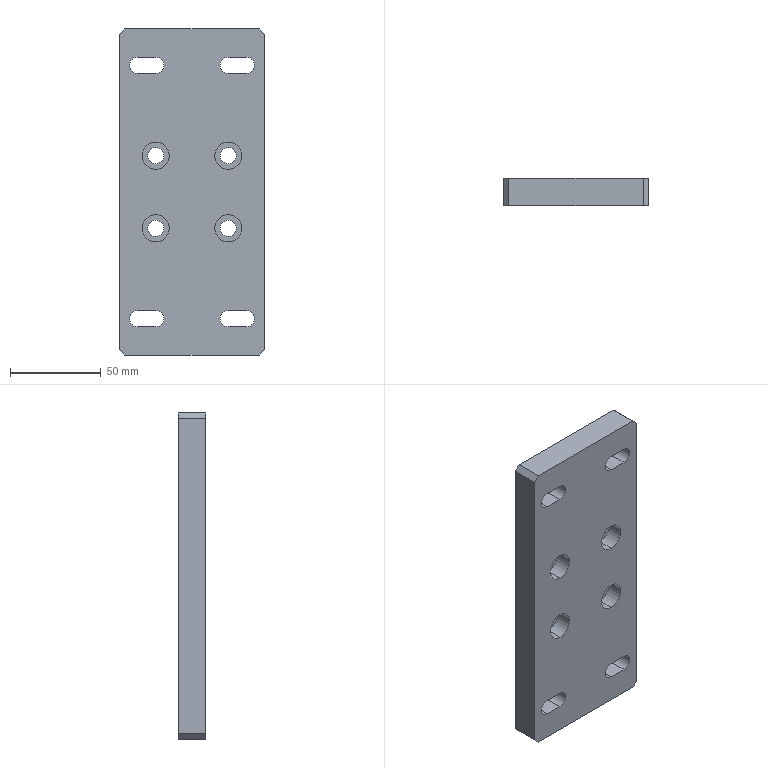Part | SolidWorks | features BaseBody 1 | 1 solid | 46 faces | box 80 x 15 x 180 mm | volume 198624 mm3 | cylinder 24 | plane 22 | commonest cylinder face diameters 9 x16 15 x8
STEP:
#1=CARTESIAN_POINT('',(-40.,7.5,87.));
#2=VERTEX_POINT('',#1);
#3=CARTESIAN_POINT('',(-37.,7.5,90.));
#4=VERTEX_POINT('',#3);
#5=CARTESIAN_POINT('',(-37.,7.5,90.));
#6=DIRECTION('',(0.7071,0.,0.7071));
#7=VECTOR('',#6,1000.);
#8=LINE('',#5,#7);
#9=EDGE_CURVE('',#2,#4,#8,.T.);
#10=ORIENTED_EDGE('',*,*,#9,.F.);
#11=CARTESIAN_POINT('',(-40.,-7.5,87.));
#12=VERTEX_POINT('',#11);
#13=CARTESIAN_POINT('',(-40.,7.5,87.));
#14=DIRECTION('',(0.,1.,0.));
#15=VECTOR('',#14,1000.);
#16=LINE('',#13,#15);
#17=EDGE_CURVE('',#12,#2,#16,.T.);
#18=ORIENTED_EDGE('',*,*,#17,.F.);
#19=CARTESIAN_POINT('',(-37.,-7.5,90.));
#20=VERTEX_POINT('',#19);
#21=CARTESIAN_POINT('',(-63.5,-7.5,63.5));
#22=DIRECTION('',(-0.7071,0.,-0.7071));
#23=VECTOR('',#22,1000.);
#24=LINE('',#21,#23);
#25=EDGE_CURVE('',#20,#12,#24,.T.);
#26=ORIENTED_EDGE('',*,*,#25,.F.);
#27=CARTESIAN_POINT('',(-37.,7.5,90.));
#28=DIRECTION('',(0.,-1.,0.));
#29=VECTOR('',#28,1000.);
#30=LINE('',#27,#29);
#31=EDGE_CURVE('',#4,#20,#30,.T.);
#32=ORIENTED_EDGE('',*,*,#31,.F.);
#33=EDGE_LOOP('',(#10,#18,#26,#32));
#34=FACE_OUTER_BOUND('',#33,.T.);
#35=CARTESIAN_POINT('',(-37.,7.5,90.));
#36=DIRECTION('',(0.7071,0.,-0.7071));
#37=DIRECTION('',(0.,-1.,0.));
#38=AXIS2_PLACEMENT_3D('',#35,#36,#37);
#39=PLANE('',#38);
#40=ADVANCED_FACE('',(#34),#39,.F.);
#41=CARTESIAN_POINT('',(-37.,7.5,-90.));
#42=VERTEX_POINT('',#41);
#43=CARTESIAN_POINT('',(-40.,7.5,-87.));
#44=VERTEX_POINT('',#43);
#45=CARTESIAN_POINT('',(-40.,7.5,-87.));
#46=DIRECTION('',(-0.7071,0.,0.7071));
#47=VECTOR('',#46,1000.);
#48=LINE('',#45,#47);
#49=EDGE_CURVE('',#42,#44,#48,.T.);
#50=ORIENTED_EDGE('',*,*,#49,.F.);
#51=CARTESIAN_POINT('',(-37.,-7.5,-90.));
#52=VERTEX_POINT('',#51);
#53=CARTESIAN_POINT('',(-37.,7.5,-90.));
#54=DIRECTION('',(0.,1.,0.));
#55=VECTOR('',#54,1000.);
#56=LINE('',#53,#55);
#57=EDGE_CURVE('',#52,#42,#56,.T.);
#58=ORIENTED_EDGE('',*,*,#57,.F.);
#59=CARTESIAN_POINT('',(-40.,-7.5,-87.));
#60=VERTEX_POINT('',#59);
#61=CARTESIAN_POINT('',(-63.5,-7.5,-63.5));
#62=DIRECTION('',(0.7071,0.,-0.7071));
#63=VECTOR('',#62,1000.);
#64=LINE('',#61,#63);
#65=EDGE_CURVE('',#60,#52,#64,.T.);
#66=ORIENTED_EDGE('',*,*,#65,.F.);
#67=CARTESIAN_POINT('',(-40.,7.5,-87.));
#68=DIRECTION('',(0.,-1.,0.));
#69=VECTOR('',#68,1000.);
#70=LINE('',#67,#69);
#71=EDGE_CURVE('',#44,#60,#70,.T.);
#72=ORIENTED_EDGE('',*,*,#71,.F.);
#73=EDGE_LOOP('',(#50,#58,#66,#72));
#74=FACE_OUTER_BOUND('',#73,.T.);
#75=CARTESIAN_POINT('',(-40.,7.5,-87.));
#76=DIRECTION('',(0.7071,0.,0.7071));
#77=DIRECTION('',(0.,-1.,0.));
#78=AXIS2_PLACEMENT_3D('',#75,#76,#77);
#79=PLANE('',#78);
#80=ADVANCED_FACE('',(#74),#79,.F.);
#81=CARTESIAN_POINT('',(37.,7.5,90.));
#82=VERTEX_POINT('',#81);
#83=CARTESIAN_POINT('',(40.,7.5,87.));
#84=VERTEX_POINT('',#83);
#85=CARTESIAN_POINT('',(40.,7.5,87.));
#86=DIRECTION('',(0.7071,0.,-0.7071));
#87=VECTOR('',#86,1000.);
#88=LINE('',#85,#87);
#89=EDGE_CURVE('',#82,#84,#88,.T.);
#90=ORIENTED_EDGE('',*,*,#89,.F.);
#91=CARTESIAN_POINT('',(37.,-7.5,90.));
#92=VERTEX_POINT('',#91);
#93=CARTESIAN_POINT('',(37.,7.5,90.));
#94=DIRECTION('',(0.,1.,0.));
#95=VECTOR('',#94,1000.);
#96=LINE('',#93,#95);
#97=EDGE_CURVE('',#92,#82,#96,.T.);
#98=ORIENTED_EDGE('',*,*,#97,.F.);
#99=CARTESIAN_POINT('',(40.,-7.5,87.));
#100=VERTEX_POINT('',#99);
#101=CARTESIAN_POINT('',(63.5,-7.5,63.5));
#102=DIRECTION('',(-0.7071,0.,0.7071));
#103=VECTOR('',#102,1000.);
#104=LINE('',#101,#103);
#105=EDGE_CURVE('',#100,#92,#104,.T.);
#106=ORIENTED_EDGE('',*,*,#105,.F.);
#107=CARTESIAN_POINT('',(40.,7.5,87.));
#108=DIRECTION('',(0.,-1.,0.));
#109=VECTOR('',#108,1000.);
#110=LINE('',#107,#109);
#111=EDGE_CURVE('',#84,#100,#110,.T.);
#112=ORIENTED_EDGE('',*,*,#111,.F.);
#113=EDGE_LOOP('',(#90,#98,#106,#112));
#114=FACE_OUTER_BOUND('',#113,.T.);
#115=CARTESIAN_POINT('',(40.,7.5,87.));
#116=DIRECTION('',(-0.7071,0.,-0.7071));
#117=DIRECTION('',(-0.7071,0.,0.7071));
#118=AXIS2_PLACEMENT_3D('',#115,#116,#117);
#119=PLANE('',#118);
#120=ADVANCED_FACE('',(#114),#119,.F.);
#121=CARTESIAN_POINT('',(40.,7.5,-87.));
#122=VERTEX_POINT('',#121);
#123=CARTESIAN_POINT('',(37.,7.5,-90.));
#124=VERTEX_POINT('',#123);
#125=CARTESIAN_POINT('',(37.,7.5,-90.));
#126=DIRECTION('',(-0.7071,0.,-0.7071));
#127=VECTOR('',#126,1000.);
#128=LINE('',#125,#127);
#129=EDGE_CURVE('',#122,#124,#128,.T.);
#130=ORIENTED_EDGE('',*,*,#129,.F.);
#131=CARTESIAN_POINT('',(40.,-7.5,-87.));
#132=VERTEX_POINT('',#131);
#133=CARTESIAN_POINT('',(40.,7.5,-87.));
#134=DIRECTION('',(0.,1.,0.));
#135=VECTOR('',#134,1000.);
#136=LINE('',#133,#135);
#137=EDGE_CURVE('',#132,#122,#136,.T.);
#138=ORIENTED_EDGE('',*,*,#137,.F.);
#139=CARTESIAN_POINT('',(37.,-7.5,-90.));
#140=VERTEX_POINT('',#139);
#141=CARTESIAN_POINT('',(63.5,-7.5,-63.5));
#142=DIRECTION('',(0.7071,0.,0.7071));
#143=VECTOR('',#142,1000.);
#144=LINE('',#141,#143);
#145=EDGE_CURVE('',#140,#132,#144,.T.);
#146=ORIENTED_EDGE('',*,*,#145,.F.);
#147=CARTESIAN_POINT('',(37.,7.5,-90.));
#148=DIRECTION('',(0.,-1.,0.));
#149=VECTOR('',#148,1000.);
#150=LINE('',#147,#149);
#151=EDGE_CURVE('',#124,#140,#150,.T.);
#152=ORIENTED_EDGE('',*,*,#151,.F.);
#153=EDGE_LOOP('',(#130,#138,#146,#152));
#154=FACE_OUTER_BOUND('',#153,.T.);
#155=CARTESIAN_POINT('',(37.,7.5,-90.));
#156=DIRECTION('',(-0.7071,0.,0.7071));
#157=DIRECTION('',(0.,1.,0.));
#158=AXIS2_PLACEMENT_3D('',#155,#156,#157);
#159=PLANE('',#158);
#160=ADVANCED_FACE('',(#154),#159,.F.);
#161=CARTESIAN_POINT('',(-20.,-7.5,74.5));
#162=VERTEX_POINT('',#161);
#163=CARTESIAN_POINT('',(-30.,-7.5,74.5));
#164=VERTEX_POINT('',#163);
#165=CARTESIAN_POINT('',(0.,-7.5,74.5));
#166=DIRECTION('',(-1.,0.,0.));
#167=VECTOR('',#166,1000.);
#168=LINE('',#165,#167);
#169=EDGE_CURVE('',#162,#164,#168,.T.);
#170=ORIENTED_EDGE('',*,*,#169,.T.);
#171=CARTESIAN_POINT('',(-30.,7.5,74.5));
#172=VERTEX_POINT('',#171);
#173=CARTESIAN_POINT('',(-30.,7.5,74.5));
#174=DIRECTION('',(0.,1.,0.));
#175=VECTOR('',#174,1000.);
#176=LINE('',#173,#175);
#177=EDGE_CURVE('',#164,#172,#176,.T.);
#178=ORIENTED_EDGE('',*,*,#177,.T.);
#179=CARTESIAN_POINT('',(-20.,7.5,74.5));
#180=VERTEX_POINT('',#179);
#181=CARTESIAN_POINT('',(-30.,7.5,74.5));
#182=DIRECTION('',(1.,0.,0.));
#183=VECTOR('',#182,1000.);
#184=LINE('',#181,#183);
#185=EDGE_CURVE('',#172,#180,#184,.T.);
#186=ORIENTED_EDGE('',*,*,#185,.T.);
#187=CARTESIAN_POINT('',(-20.,7.5,74.5));
#188=DIRECTION('',(0.,-1.,0.));
#189=VECTOR('',#188,1000.);
#190=LINE('',#187,#189);
#191=EDGE_CURVE('',#180,#162,#190,.T.);
#192=ORIENTED_EDGE('',*,*,#191,.T.);
#193=EDGE_LOOP('',(#170,#178,#186,#192));
#194=FACE_OUTER_BOUND('',#193,.T.);
#195=CARTESIAN_POINT('',(-30.,7.5,74.5));
#196=DIRECTION('',(0.,0.,1.));
#197=DIRECTION('',(1.,0.,0.));
#198=AXIS2_PLACEMENT_3D('',#195,#196,#197);
#199=PLANE('',#198);
#200=ADVANCED_FACE('',(#194),#199,.F.);
#201=CARTESIAN_POINT('',(-30.,-7.5,65.5));
#202=VERTEX_POINT('',#201);
#203=CARTESIAN_POINT('',(-20.,-7.5,65.5));
#204=VERTEX_POINT('',#203);
#205=CARTESIAN_POINT('',(0.,-7.5,65.5));
#206=DIRECTION('',(1.,0.,0.));
#207=VECTOR('',#206,1000.);
#208=LINE('',#205,#207);
#209=EDGE_CURVE('',#202,#204,#208,.T.);
#210=ORIENTED_EDGE('',*,*,#209,.T.);
#211=CARTESIAN_POINT('',(-20.,7.5,65.5));
#212=VERTEX_POINT('',#211);
#213=CARTESIAN_POINT('',(-20.,7.5,65.5));
#214=DIRECTION('',(0.,1.,0.));
#215=VECTOR('',#214,1000.);
#216=LINE('',#213,#215);
#217=EDGE_CURVE('',#204,#212,#216,.T.);
#218=ORIENTED_EDGE('',*,*,#217,.T.);
#219=CARTESIAN_POINT('',(-30.,7.5,65.5));
#220=VERTEX_POINT('',#219);
#221=CARTESIAN_POINT('',(-30.,7.5,65.5));
#222=DIRECTION('',(1.,0.,0.));
#223=VECTOR('',#222,1000.);
#224=LINE('',#221,#223);
#225=EDGE_CURVE('',#220,#212,#224,.T.);
#226=ORIENTED_EDGE('',*,*,#225,.F.);
#227=CARTESIAN_POINT('',(-30.,7.5,65.5));
#228=DIRECTION('',(0.,-1.,0.));
#229=VECTOR('',#228,1000.);
#230=LINE('',#227,#229);
#231=EDGE_CURVE('',#220,#202,#230,.T.);
#232=ORIENTED_EDGE('',*,*,#231,.T.);
#233=EDGE_LOOP('',(#210,#218,#226,#232));
#234=FACE_OUTER_BOUND('',#233,.T.);
#235=CARTESIAN_POINT('',(-30.,7.5,65.5));
#236=DIRECTION('',(0.,0.,-1.));
#237=DIRECTION('',(0.,-1.,0.));
#238=AXIS2_PLACEMENT_3D('',#235,#236,#237);
#239=PLANE('',#238);
#240=ADVANCED_FACE('',(#234),#239,.F.);
#241=CARTESIAN_POINT('',(-30.,-7.5,70.));
#242=DIRECTION('',(0.,-1.,0.));
#243=DIRECTION('',(0.,0.,-1.));
#244=AXIS2_PLACEMENT_3D('',#241,#242,#243);
#245=CIRCLE('',#244,4.5);
#246=EDGE_CURVE('',#164,#202,#245,.T.);
#247=ORIENTED_EDGE('',*,*,#246,.T.);
#248=ORIENTED_EDGE('',*,*,#231,.F.);
#249=CARTESIAN_POINT('',(-30.,7.5,70.));
#250=DIRECTION('',(0.,1.,0.));
#251=DIRECTION('',(0.,0.,1.));
#252=AXIS2_PLACEMENT_3D('',#249,#250,#251);
#253=CIRCLE('',#252,4.5);
#254=EDGE_CURVE('',#220,#172,#253,.T.);
#255=ORIENTED_EDGE('',*,*,#254,.T.);
#256=ORIENTED_EDGE('',*,*,#177,.F.);
#257=EDGE_LOOP('',(#247,#248,#255,#256));
#258=FACE_OUTER_BOUND('',#257,.T.);
#259=CARTESIAN_POINT('',(-30.,7.5,70.));
#260=DIRECTION('',(0.,1.,0.));
#261=DIRECTION('',(0.,0.,1.));
#262=AXIS2_PLACEMENT_3D('',#259,#260,#261);
#263=CYLINDRICAL_SURFACE('',#262,4.5);
#264=ADVANCED_FACE('',(#258),#263,.F.);
#265=CARTESIAN_POINT('',(-20.,-7.5,70.));
#266=DIRECTION('',(0.,-1.,0.));
#267=DIRECTION('',(0.,0.,-1.));
#268=AXIS2_PLACEMENT_3D('',#265,#266,#267);
#269=CIRCLE('',#268,4.5);
#270=EDGE_CURVE('',#204,#162,#269,.T.);
#271=ORIENTED_EDGE('',*,*,#270,.T.);
#272=ORIENTED_EDGE('',*,*,#191,.F.);
#273=CARTESIAN_POINT('',(-20.,7.5,70.));
#274=DIRECTION('',(0.,1.,0.));
#275=DIRECTION('',(0.,0.,1.));
#276=AXIS2_PLACEMENT_3D('',#273,#274,#275);
#277=CIRCLE('',#276,4.5);
#278=EDGE_CURVE('',#180,#212,#277,.T.);
#279=ORIENTED_EDGE('',*,*,#278,.T.);
#280=ORIENTED_EDGE('',*,*,#217,.F.);
#281=EDGE_LOOP('',(#271,#272,#279,#280));
#282=FACE_OUTER_BOUND('',#281,.T.);
#283=CARTESIAN_POINT('',(-20.,7.5,70.));
#284=DIRECTION('',(0.,1.,0.));
#285=DIRECTION('',(0.,0.,1.));
#286=AXIS2_PLACEMENT_3D('',#283,#284,#285);
#287=CYLINDRICAL_SURFACE('',#286,4.5);
#288=ADVANCED_FACE('',(#282),#287,.F.);
#289=CARTESIAN_POINT('',(30.,-7.5,74.5));
#290=VERTEX_POINT('',#289);
#291=CARTESIAN_POINT('',(20.,-7.5,74.5));
#292=VERTEX_POINT('',#291);
#293=CARTESIAN_POINT('',(0.,-7.5,74.5));
#294=DIRECTION('',(-1.,0.,0.));
#295=VECTOR('',#294,1000.);
#296=LINE('',#293,#295);
#297=EDGE_CURVE('',#290,#292,#296,.T.);
#298=ORIENTED_EDGE('',*,*,#297,.T.);
#299=CARTESIAN_POINT('',(20.,7.5,74.5));
#300=VERTEX_POINT('',#299);
#301=CARTESIAN_POINT('',(20.,7.5,74.5));
#302=DIRECTION('',(0.,1.,0.));
#303=VECTOR('',#302,1000.);
#304=LINE('',#301,#303);
#305=EDGE_CURVE('',#292,#300,#304,.T.);
#306=ORIENTED_EDGE('',*,*,#305,.T.);
#307=CARTESIAN_POINT('',(30.,7.5,74.5));
#308=VERTEX_POINT('',#307);
#309=CARTESIAN_POINT('',(20.,7.5,74.5));
#310=DIRECTION('',(1.,0.,0.));
#311=VECTOR('',#310,1000.);
#312=LINE('',#309,#311);
#313=EDGE_CURVE('',#300,#308,#312,.T.);
#314=ORIENTED_EDGE('',*,*,#313,.T.);
#315=CARTESIAN_POINT('',(30.,7.5,74.5));
#316=DIRECTION('',(0.,-1.,0.));
#317=VECTOR('',#316,1000.);
#318=LINE('',#315,#317);
#319=EDGE_CURVE('',#308,#290,#318,.T.);
#320=ORIENTED_EDGE('',*,*,#319,.T.);
#321=EDGE_LOOP('',(#298,#306,#314,#320));
#322=FACE_OUTER_BOUND('',#321,.T.);
#323=CARTESIAN_POINT('',(20.,7.5,74.5));
#324=DIRECTION('',(0.,0.,1.));
#325=DIRECTION('',(1.,0.,0.));
#326=AXIS2_PLACEMENT_3D('',#323,#324,#325);
#327=PLANE('',#326);
#328=ADVANCED_FACE('',(#322),#327,.F.);
#329=CARTESIAN_POINT('',(20.,-7.5,65.5));
#330=VERTEX_POINT('',#329);
#331=CARTESIAN_POINT('',(30.,-7.5,65.5));
#332=VERTEX_POINT('',#331);
#333=CARTESIAN_POINT('',(0.,-7.5,65.5));
#334=DIRECTION('',(1.,0.,0.));
#335=VECTOR('',#334,1000.);
#336=LINE('',#333,#335);
#337=EDGE_CURVE('',#330,#332,#336,.T.);
#338=ORIENTED_EDGE('',*,*,#337,.T.);
#339=CARTESIAN_POINT('',(30.,7.5,65.5));
#340=VERTEX_POINT('',#339);
#341=CARTESIAN_POINT('',(30.,7.5,65.5));
#342=DIRECTION('',(0.,1.,0.));
#343=VECTOR('',#342,1000.);
#344=LINE('',#341,#343);
#345=EDGE_CURVE('',#332,#340,#344,.T.);
#346=ORIENTED_EDGE('',*,*,#345,.T.);
#347=CARTESIAN_POINT('',(20.,7.5,65.5));
#348=VERTEX_POINT('',#347);
#349=CARTESIAN_POINT('',(20.,7.5,65.5));
#350=DIRECTION('',(1.,0.,0.));
#351=VECTOR('',#350,1000.);
#352=LINE('',#349,#351);
#353=EDGE_CURVE('',#348,#340,#352,.T.);
#354=ORIENTED_EDGE('',*,*,#353,.F.);
#355=CARTESIAN_POINT('',(20.,7.5,65.5));
#356=DIRECTION('',(0.,-1.,0.));
#357=VECTOR('',#356,1000.);
#358=LINE('',#355,#357);
#359=EDGE_CURVE('',#348,#330,#358,.T.);
#360=ORIENTED_EDGE('',*,*,#359,.T.);
#361=EDGE_LOOP('',(#338,#346,#354,#360));
#362=FACE_OUTER_BOUND('',#361,.T.);
#363=CARTESIAN_POINT('',(20.,7.5,65.5));
#364=DIRECTION('',(0.,0.,-1.));
#365=DIRECTION('',(0.,-1.,0.));
#366=AXIS2_PLACEMENT_3D('',#363,#364,#365);
#367=PLANE('',#366);
#368=ADVANCED_FACE('',(#362),#367,.F.);
#369=CARTESIAN_POINT('',(20.,-7.5,70.));
#370=DIRECTION('',(0.,-1.,0.));
#371=DIRECTION('',(0.,0.,-1.));
#372=AXIS2_PLACEMENT_3D('',#369,#370,#371);
#373=CIRCLE('',#372,4.5);
#374=EDGE_CURVE('',#292,#330,#373,.T.);
#375=ORIENTED_EDGE('',*,*,#374,.T.);
#376=ORIENTED_EDGE('',*,*,#359,.F.);
#377=CARTESIAN_POINT('',(20.,7.5,70.));
#378=DIRECTION('',(0.,1.,0.));
#379=DIRECTION('',(0.,0.,1.));
#380=AXIS2_PLACEMENT_3D('',#377,#378,#379);
#381=CIRCLE('',#380,4.5);
#382=EDGE_CURVE('',#348,#300,#381,.T.);
#383=ORIENTED_EDGE('',*,*,#382,.T.);
#384=ORIENTED_EDGE('',*,*,#305,.F.);
#385=EDGE_LOOP('',(#375,#376,#383,#384));
#386=FACE_OUTER_BOUND('',#385,.T.);
#387=CARTESIAN_POINT('',(20.,7.5,70.));
#388=DIRECTION('',(0.,1.,0.));
#389=DIRECTION('',(0.,0.,1.));
#390=AXIS2_PLACEMENT_3D('',#387,#388,#389);
#391=CYLINDRICAL_SURFACE('',#390,4.5);
#392=ADVANCED_FACE('',(#386),#391,.F.);
#393=CARTESIAN_POINT('',(30.,-7.5,70.));
#394=DIRECTION('',(0.,-1.,0.));
#395=DIRECTION('',(0.,0.,-1.));
#396=AXIS2_PLACEMENT_3D('',#393,#394,#395);
#397=CIRCLE('',#396,4.5);
#398=EDGE_CURVE('',#332,#290,#397,.T.);
#399=ORIENTED_EDGE('',*,*,#398,.T.);
#400=ORIENTED_EDGE('',*,*,#319,.F.);
#401=CARTESIAN_POINT('',(30.,7.5,70.));
#402=DIRECTION('',(0.,1.,0.));
#403=DIRECTION('',(0.,0.,1.));
#404=AXIS2_PLACEMENT_3D('',#401,#402,#403);
#405=CIRCLE('',#404,4.5);
#406=EDGE_CURVE('',#308,#340,#405,.T.);
#407=ORIENTED_EDGE('',*,*,#406,.T.);
#408=ORIENTED_EDGE('',*,*,#345,.F.);
#409=EDGE_LOOP('',(#399,#400,#407,#408));
#410=FACE_OUTER_BOUND('',#409,.T.);
#411=CARTESIAN_POINT('',(30.,7.5,70.));
#412=DIRECTION('',(0.,1.,0.));
#413=DIRECTION('',(0.,0.,1.));
#414=AXIS2_PLACEMENT_3D('',#411,#412,#413);
#415=CYLINDRICAL_SURFACE('',#414,4.5);
#416=ADVANCED_FACE('',(#410),#415,.F.);
#417=CARTESIAN_POINT('',(30.,-7.5,-65.5));
#418=VERTEX_POINT('',#417);
#419=CARTESIAN_POINT('',(20.,-7.5,-65.5));
#420=VERTEX_POINT('',#419);
#421=CARTESIAN_POINT('',(0.,-7.5,-65.5));
#422=DIRECTION('',(-1.,0.,0.));
#423=VECTOR('',#422,1000.);
#424=LINE('',#421,#423);
#425=EDGE_CURVE('',#418,#420,#424,.T.);
#426=ORIENTED_EDGE('',*,*,#425,.T.);
#427=CARTESIAN_POINT('',(20.,7.5,-65.5));
#428=VERTEX_POINT('',#427);
#429=CARTESIAN_POINT('',(20.,7.5,-65.5));
#430=DIRECTION('',(0.,1.,0.));
#431=VECTOR('',#430,1000.);
#432=LINE('',#429,#431);
#433=EDGE_CURVE('',#420,#428,#432,.T.);
#434=ORIENTED_EDGE('',*,*,#433,.T.);
#435=CARTESIAN_POINT('',(30.,7.5,-65.5));
#436=VERTEX_POINT('',#435);
#437=CARTESIAN_POINT('',(20.,7.5,-65.5));
#438=DIRECTION('',(1.,0.,0.));
#439=VECTOR('',#438,1000.);
#440=LINE('',#437,#439);
#441=EDGE_CURVE('',#428,#436,#440,.T.);
#442=ORIENTED_EDGE('',*,*,#441,.T.);
#443=CARTESIAN_POINT('',(30.,7.5,-65.5));
#444=DIRECTION('',(0.,-1.,0.));
#445=VECTOR('',#444,1000.);
#446=LINE('',#443,#445);
#447=EDGE_CURVE('',#436,#418,#446,.T.);
#448=ORIENTED_EDGE('',*,*,#447,.T.);
#449=EDGE_LOOP('',(#426,#434,#442,#448));
#450=FACE_OUTER_BOUND('',#449,.T.);
#451=CARTESIAN_POINT('',(20.,7.5,-65.5));
#452=DIRECTION('',(0.,0.,1.));
#453=DIRECTION('',(1.,0.,0.));
#454=AXIS2_PLACEMENT_3D('',#451,#452,#453);
#455=PLANE('',#454);
#456=ADVANCED_FACE('',(#450),#455,.F.);
#457=CARTESIAN_POINT('',(20.,-7.5,-74.5));
#458=VERTEX_POINT('',#457);
#459=CARTESIAN_POINT('',(30.,-7.5,-74.5));
#460=VERTEX_POINT('',#459);
#461=CARTESIAN_POINT('',(0.,-7.5,-74.5));
#462=DIRECTION('',(1.,0.,0.));
#463=VECTOR('',#462,1000.);
#464=LINE('',#461,#463);
#465=EDGE_CURVE('',#458,#460,#464,.T.);
#466=ORIENTED_EDGE('',*,*,#465,.T.);
#467=CARTESIAN_POINT('',(30.,7.5,-74.5));
#468=VERTEX_POINT('',#467);
#469=CARTESIAN_POINT('',(30.,7.5,-74.5));
#470=DIRECTION('',(0.,1.,0.));
#471=VECTOR('',#470,1000.);
#472=LINE('',#469,#471);
#473=EDGE_CURVE('',#460,#468,#472,.T.);
#474=ORIENTED_EDGE('',*,*,#473,.T.);
#475=CARTESIAN_POINT('',(20.,7.5,-74.5));
#476=VERTEX_POINT('',#475);
#477=CARTESIAN_POINT('',(20.,7.5,-74.5));
#478=DIRECTION('',(1.,0.,0.));
#479=VECTOR('',#478,1000.);
#480=LINE('',#477,#479);
#481=EDGE_CURVE('',#476,#468,#480,.T.);
#482=ORIENTED_EDGE('',*,*,#481,.F.);
#483=CARTESIAN_POINT('',(20.,7.5,-74.5));
#484=DIRECTION('',(0.,-1.,0.));
#485=VECTOR('',#484,1000.);
#486=LINE('',#483,#485);
#487=EDGE_CURVE('',#476,#458,#486,.T.);
#488=ORIENTED_EDGE('',*,*,#487,.T.);
#489=EDGE_LOOP('',(#466,#474,#482,#488));
#490=FACE_OUTER_BOUND('',#489,.T.);
#491=CARTESIAN_POINT('',(20.,7.5,-74.5));
#492=DIRECTION('',(0.,0.,-1.));
#493=DIRECTION('',(0.,-1.,0.));
#494=AXIS2_PLACEMENT_3D('',#491,#492,#493);
#495=PLANE('',#494);
#496=ADVANCED_FACE('',(#490),#495,.F.);
#497=CARTESIAN_POINT('',(20.,-7.5,-70.));
#498=DIRECTION('',(0.,-1.,0.));
#499=DIRECTION('',(0.,0.,-1.));
#500=AXIS2_PLACEMENT_3D('',#497,#498,#499);
#501=CIRCLE('',#500,4.5);
#502=EDGE_CURVE('',#420,#458,#501,.T.);
#503=ORIENTED_EDGE('',*,*,#502,.T.);
#504=ORIENTED_EDGE('',*,*,#487,.F.);
#505=CARTESIAN_POINT('',(20.,7.5,-70.));
#506=DIRECTION('',(0.,1.,0.));
#507=DIRECTION('',(0.,0.,1.));
#508=AXIS2_PLACEMENT_3D('',#505,#506,#507);
#509=CIRCLE('',#508,4.5);
#510=EDGE_CURVE('',#476,#428,#509,.T.);
#511=ORIENTED_EDGE('',*,*,#510,.T.);
#512=ORIENTED_EDGE('',*,*,#433,.F.);
#513=EDGE_LOOP('',(#503,#504,#511,#512));
#514=FACE_OUTER_BOUND('',#513,.T.);
#515=CARTESIAN_POINT('',(20.,7.5,-70.));
#516=DIRECTION('',(0.,1.,0.));
#517=DIRECTION('',(0.,0.,1.));
#518=AXIS2_PLACEMENT_3D('',#515,#516,#517);
#519=CYLINDRICAL_SURFACE('',#518,4.5);
#520=ADVANCED_FACE('',(#514),#519,.F.);
#521=CARTESIAN_POINT('',(30.,-7.5,-70.));
#522=DIRECTION('',(0.,-1.,0.));
#523=DIRECTION('',(0.,0.,-1.));
#524=AXIS2_PLACEMENT_3D('',#521,#522,#523);
#525=CIRCLE('',#524,4.5);
#526=EDGE_CURVE('',#460,#418,#525,.T.);
#527=ORIENTED_EDGE('',*,*,#526,.T.);
#528=ORIENTED_EDGE('',*,*,#447,.F.);
#529=CARTESIAN_POINT('',(30.,7.5,-70.));
#530=DIRECTION('',(0.,1.,0.));
#531=DIRECTION('',(0.,0.,1.));
#532=AXIS2_PLACEMENT_3D('',#529,#530,#531);
#533=CIRCLE('',#532,4.5);
#534=EDGE_CURVE('',#436,#468,#533,.T.);
#535=ORIENTED_EDGE('',*,*,#534,.T.);
#536=ORIENTED_EDGE('',*,*,#473,.F.);
#537=EDGE_LOOP('',(#527,#528,#535,#536));
#538=FACE_OUTER_BOUND('',#537,.T.);
#539=CARTESIAN_POINT('',(30.,7.5,-70.));
#540=DIRECTION('',(0.,1.,0.));
#541=DIRECTION('',(0.,0.,1.));
#542=AXIS2_PLACEMENT_3D('',#539,#540,#541);
#543=CYLINDRICAL_SURFACE('',#542,4.5);
#544=ADVANCED_FACE('',(#538),#543,.F.);
#545=CARTESIAN_POINT('',(-20.,-7.5,-65.5));
#546=VERTEX_POINT('',#545);
#547=CARTESIAN_POINT('',(-30.,-7.5,-65.5));
#548=VERTEX_POINT('',#547);
#549=CARTESIAN_POINT('',(0.,-7.5,-65.5));
#550=DIRECTION('',(-1.,0.,0.));
#551=VECTOR('',#550,1000.);
#552=LINE('',#549,#551);
#553=EDGE_CURVE('',#546,#548,#552,.T.);
#554=ORIENTED_EDGE('',*,*,#553,.T.);
#555=CARTESIAN_POINT('',(-30.,7.5,-65.5));
#556=VERTEX_POINT('',#555);
#557=CARTESIAN_POINT('',(-30.,7.5,-65.5));
#558=DIRECTION('',(0.,1.,0.));
#559=VECTOR('',#558,1000.);
#560=LINE('',#557,#559);
#561=EDGE_CURVE('',#548,#556,#560,.T.);
#562=ORIENTED_EDGE('',*,*,#561,.T.);
#563=CARTESIAN_POINT('',(-20.,7.5,-65.5));
#564=VERTEX_POINT('',#563);
#565=CARTESIAN_POINT('',(-30.,7.5,-65.5));
#566=DIRECTION('',(1.,0.,0.));
#567=VECTOR('',#566,1000.);
#568=LINE('',#565,#567);
#569=EDGE_CURVE('',#556,#564,#568,.T.);
#570=ORIENTED_EDGE('',*,*,#569,.T.);
#571=CARTESIAN_POINT('',(-20.,7.5,-65.5));
#572=DIRECTION('',(0.,-1.,0.));
#573=VECTOR('',#572,1000.);
#574=LINE('',#571,#573);
#575=EDGE_CURVE('',#564,#546,#574,.T.);
#576=ORIENTED_EDGE('',*,*,#575,.T.);
#577=EDGE_LOOP('',(#554,#562,#570,#576));
#578=FACE_OUTER_BOUND('',#577,.T.);
#579=CARTESIAN_POINT('',(-30.,7.5,-65.5));
#580=DIRECTION('',(0.,0.,1.));
#581=DIRECTION('',(1.,0.,0.));
#582=AXIS2_PLACEMENT_3D('',#579,#580,#581);
#583=PLANE('',#582);
#584=ADVANCED_FACE('',(#578),#583,.F.);
#585=CARTESIAN_POINT('',(-30.,-7.5,-74.5));
#586=VERTEX_POINT('',#585);
#587=CARTESIAN_POINT('',(-20.,-7.5,-74.5));
#588=VERTEX_POINT('',#587);
#589=CARTESIAN_POINT('',(0.,-7.5,-74.5));
#590=DIRECTION('',(1.,0.,0.));
#591=VECTOR('',#590,1000.);
#592=LINE('',#589,#591);
#593=EDGE_CURVE('',#586,#588,#592,.T.);
#594=ORIENTED_EDGE('',*,*,#593,.T.);
#595=CARTESIAN_POINT('',(-20.,7.5,-74.5));
#596=VERTEX_POINT('',#595);
#597=CARTESIAN_POINT('',(-20.,7.5,-74.5));
#598=DIRECTION('',(0.,1.,0.));
#599=VECTOR('',#598,1000.);
#600=LINE('',#597,#599);
#601=EDGE_CURVE('',#588,#596,#600,.T.);
#602=ORIENTED_EDGE('',*,*,#601,.T.);
#603=CARTESIAN_POINT('',(-30.,7.5,-74.5));
#604=VERTEX_POINT('',#603);
#605=CARTESIAN_POINT('',(-30.,7.5,-74.5));
#606=DIRECTION('',(1.,0.,0.));
#607=VECTOR('',#606,1000.);
#608=LINE('',#605,#607);
#609=EDGE_CURVE('',#604,#596,#608,.T.);
#610=ORIENTED_EDGE('',*,*,#609,.F.);
#611=CARTESIAN_POINT('',(-30.,7.5,-74.5));
#612=DIRECTION('',(0.,-1.,0.));
#613=VECTOR('',#612,1000.);
#614=LINE('',#611,#613);
#615=EDGE_CURVE('',#604,#586,#614,.T.);
#616=ORIENTED_EDGE('',*,*,#615,.T.);
#617=EDGE_LOOP('',(#594,#602,#610,#616));
#618=FACE_OUTER_BOUND('',#617,.T.);
#619=CARTESIAN_POINT('',(-30.,7.5,-74.5));
#620=DIRECTION('',(0.,0.,-1.));
#621=DIRECTION('',(0.,-1.,0.));
#622=AXIS2_PLACEMENT_3D('',#619,#620,#621);
#623=PLANE('',#622);
#624=ADVANCED_FACE('',(#618),#623,.F.);
#625=CARTESIAN_POINT('',(-30.,-7.5,-70.));
#626=DIRECTION('',(0.,-1.,0.));
#627=DIRECTION('',(0.,0.,-1.));
#628=AXIS2_PLACEMENT_3D('',#625,#626,#627);
#629=CIRCLE('',#628,4.5);
#630=EDGE_CURVE('',#548,#586,#629,.T.);
#631=ORIENTED_EDGE('',*,*,#630,.T.);
#632=ORIENTED_EDGE('',*,*,#615,.F.);
#633=CARTESIAN_POINT('',(-30.,7.5,-70.));
#634=DIRECTION('',(0.,1.,0.));
#635=DIRECTION('',(0.,0.,1.));
#636=AXIS2_PLACEMENT_3D('',#633,#634,#635);
#637=CIRCLE('',#636,4.5);
#638=EDGE_CURVE('',#604,#556,#637,.T.);
#639=ORIENTED_EDGE('',*,*,#638,.T.);
#640=ORIENTED_EDGE('',*,*,#561,.F.);
#641=EDGE_LOOP('',(#631,#632,#639,#640));
#642=FACE_OUTER_BOUND('',#641,.T.);
#643=CARTESIAN_POINT('',(-30.,7.5,-70.));
#644=DIRECTION('',(0.,1.,0.));
#645=DIRECTION('',(0.,0.,1.));
#646=AXIS2_PLACEMENT_3D('',#643,#644,#645);
#647=CYLINDRICAL_SURFACE('',#646,4.5);
#648=ADVANCED_FACE('',(#642),#647,.F.);
#649=CARTESIAN_POINT('',(-20.,-7.5,-70.));
#650=DIRECTION('',(0.,-1.,0.));
#651=DIRECTION('',(0.,0.,-1.));
#652=AXIS2_PLACEMENT_3D('',#649,#650,#651);
#653=CIRCLE('',#652,4.5);
#654=EDGE_CURVE('',#588,#546,#653,.T.);
#655=ORIENTED_EDGE('',*,*,#654,.T.);
#656=ORIENTED_EDGE('',*,*,#575,.F.);
#657=CARTESIAN_POINT('',(-20.,7.5,-70.));
#658=DIRECTION('',(0.,1.,0.));
#659=DIRECTION('',(0.,0.,1.));
#660=AXIS2_PLACEMENT_3D('',#657,#658,#659);
#661=CIRCLE('',#660,4.5);
#662=EDGE_CURVE('',#564,#596,#661,.T.);
#663=ORIENTED_EDGE('',*,*,#662,.T.);
#664=ORIENTED_EDGE('',*,*,#601,.F.);
#665=EDGE_LOOP('',(#655,#656,#663,#664));
#666=FACE_OUTER_BOUND('',#665,.T.);
#667=CARTESIAN_POINT('',(-20.,7.5,-70.));
#668=DIRECTION('',(0.,1.,0.));
#669=DIRECTION('',(0.,0.,1.));
#670=AXIS2_PLACEMENT_3D('',#667,#668,#669);
#671=CYLINDRICAL_SURFACE('',#670,4.5);
#672=ADVANCED_FACE('',(#666),#671,.F.);
#673=CARTESIAN_POINT('',(20.,1.5,-12.5));
#674=VERTEX_POINT('',#673);
#675=CARTESIAN_POINT('',(20.,-7.5,-12.5));
#676=VERTEX_POINT('',#675);
#677=CARTESIAN_POINT('',(20.,-7.5,-12.5));
#678=DIRECTION('',(0.,-1.,0.));
#679=VECTOR('',#678,1000.);
#680=LINE('',#677,#679);
#681=EDGE_CURVE('',#674,#676,#680,.T.);
#682=ORIENTED_EDGE('',*,*,#681,.F.);
#683=CARTESIAN_POINT('',(20.,1.5,-27.5));
#684=VERTEX_POINT('',#683);
#685=CARTESIAN_POINT('',(20.,1.5,-20.));
#686=DIRECTION('',(0.,-1.,0.));
#687=DIRECTION('',(0.,0.,-1.));
#688=AXIS2_PLACEMENT_3D('',#685,#686,#687);
#689=CIRCLE('',#688,7.5);
#690=EDGE_CURVE('',#684,#674,#689,.T.);
#691=ORIENTED_EDGE('',*,*,#690,.F.);
#692=CARTESIAN_POINT('',(20.,-7.5,-27.5));
#693=VERTEX_POINT('',#692);
#694=CARTESIAN_POINT('',(20.,-7.5,-27.5));
#695=DIRECTION('',(0.,-1.,0.));
#696=VECTOR('',#695,1000.);
#697=LINE('',#694,#696);
#698=EDGE_CURVE('',#684,#693,#697,.T.);
#699=ORIENTED_EDGE('',*,*,#698,.T.);
#700=CARTESIAN_POINT('',(20.,-7.5,-20.));
#701=DIRECTION('',(0.,-1.,0.));
#702=DIRECTION('',(0.,0.,-1.));
#703=AXIS2_PLACEMENT_3D('',#700,#701,#702);
#704=CIRCLE('',#703,7.5);
#705=EDGE_CURVE('',#693,#676,#704,.T.);
#706=ORIENTED_EDGE('',*,*,#705,.T.);
#707=EDGE_LOOP('',(#682,#691,#699,#706));
#708=FACE_OUTER_BOUND('',#707,.T.);
#709=CARTESIAN_POINT('',(20.,-7.5,-20.));
#710=DIRECTION('',(0.,-1.,0.));
#711=DIRECTION('',(0.,0.,-1.));
#712=AXIS2_PLACEMENT_3D('',#709,#710,#711);
#713=CYLINDRICAL_SURFACE('',#712,7.5);
#714=ADVANCED_FACE('',(#708),#713,.F.);
#715=CARTESIAN_POINT('',(20.,1.5,-24.5));
#716=VERTEX_POINT('',#715);
#717=CARTESIAN_POINT('',(20.,1.5,-15.5));
#718=VERTEX_POINT('',#717);
#719=CARTESIAN_POINT('',(20.,1.5,-20.));
#720=DIRECTION('',(0.,-1.,0.));
#721=DIRECTION('',(0.,0.,-1.));
#722=AXIS2_PLACEMENT_3D('',#719,#720,#721);
#723=CIRCLE('',#722,4.5);
#724=EDGE_CURVE('',#716,#718,#723,.T.);
#725=ORIENTED_EDGE('',*,*,#724,.F.);
#726=CARTESIAN_POINT('',(20.,1.5,-20.));
#727=DIRECTION('',(0.,-1.,0.));
#728=DIRECTION('',(0.,0.,-1.));
#729=AXIS2_PLACEMENT_3D('',#726,#727,#728);
#730=CIRCLE('',#729,4.5);
#731=EDGE_CURVE('',#718,#716,#730,.T.);
#732=ORIENTED_EDGE('',*,*,#731,.F.);
#733=EDGE_LOOP('',(#725,#732));
#734=FACE_BOUND('',#733,.T.);
#735=ORIENTED_EDGE('',*,*,#690,.T.);
#736=CARTESIAN_POINT('',(20.,1.5,-20.));
#737=DIRECTION('',(0.,-1.,0.));
#738=DIRECTION('',(0.,0.,-1.));
#739=AXIS2_PLACEMENT_3D('',#736,#737,#738);
#740=CIRCLE('',#739,7.5);
#741=EDGE_CURVE('',#674,#684,#740,.T.);
#742=ORIENTED_EDGE('',*,*,#741,.T.);
#743=EDGE_LOOP('',(#735,#742));
#744=FACE_OUTER_BOUND('',#743,.T.);
#745=CARTESIAN_POINT('',(24.5,1.5,-20.));
#746=DIRECTION('',(0.,1.,0.));
#747=DIRECTION('',(1.,0.,0.));
#748=AXIS2_PLACEMENT_3D('',#745,#746,#747);
#749=PLANE('',#748);
#750=ADVANCED_FACE('',(#734,#744),#749,.F.);
#751=CARTESIAN_POINT('',(20.,7.5,-15.5));
#752=VERTEX_POINT('',#751);
#753=CARTESIAN_POINT('',(20.,-7.5,-15.5));
#754=DIRECTION('',(0.,-1.,0.));
#755=VECTOR('',#754,1000.);
#756=LINE('',#753,#755);
#757=EDGE_CURVE('',#752,#718,#756,.T.);
#758=ORIENTED_EDGE('',*,*,#757,.F.);
#759=CARTESIAN_POINT('',(20.,7.5,-24.5));
#760=VERTEX_POINT('',#759);
#761=CARTESIAN_POINT('',(20.,7.5,-20.));
#762=DIRECTION('',(0.,-1.,0.));
#763=DIRECTION('',(0.,0.,-1.));
#764=AXIS2_PLACEMENT_3D('',#761,#762,#763);
#765=CIRCLE('',#764,4.5);
#766=EDGE_CURVE('',#760,#752,#765,.T.);
#767=ORIENTED_EDGE('',*,*,#766,.F.);
#768=CARTESIAN_POINT('',(20.,-7.5,-24.5));
#769=DIRECTION('',(0.,-1.,0.));
#770=VECTOR('',#769,1000.);
#771=LINE('',#768,#770);
#772=EDGE_CURVE('',#760,#716,#771,.T.);
#773=ORIENTED_EDGE('',*,*,#772,.T.);
#774=ORIENTED_EDGE('',*,*,#724,.T.);
#775=EDGE_LOOP('',(#758,#767,#773,#774));
#776=FACE_OUTER_BOUND('',#775,.T.);
#777=CARTESIAN_POINT('',(20.,-7.5,-20.));
#778=DIRECTION('',(0.,-1.,0.));
#779=DIRECTION('',(0.,0.,-1.));
#780=AXIS2_PLACEMENT_3D('',#777,#778,#779);
#781=CYLINDRICAL_SURFACE('',#780,4.5);
#782=ADVANCED_FACE('',(#776),#781,.F.);
#783=CARTESIAN_POINT('',(20.,1.5,27.5));
#784=VERTEX_POINT('',#783);
#785=CARTESIAN_POINT('',(20.,-7.5,27.5));
#786=VERTEX_POINT('',#785);
#787=CARTESIAN_POINT('',(20.,-7.5,27.5));
#788=DIRECTION('',(0.,-1.,0.));
#789=VECTOR('',#788,1000.);
#790=LINE('',#787,#789);
#791=EDGE_CURVE('',#784,#786,#790,.T.);
#792=ORIENTED_EDGE('',*,*,#791,.F.);
#793=CARTESIAN_POINT('',(20.,1.5,12.5));
#794=VERTEX_POINT('',#793);
#795=CARTESIAN_POINT('',(20.,1.5,20.));
#796=DIRECTION('',(0.,-1.,0.));
#797=DIRECTION('',(0.,0.,-1.));
#798=AXIS2_PLACEMENT_3D('',#795,#796,#797);
#799=CIRCLE('',#798,7.5);
#800=EDGE_CURVE('',#794,#784,#799,.T.);
#801=ORIENTED_EDGE('',*,*,#800,.F.);
#802=CARTESIAN_POINT('',(20.,-7.5,12.5));
#803=VERTEX_POINT('',#802);
#804=CARTESIAN_POINT('',(20.,-7.5,12.5));
#805=DIRECTION('',(0.,-1.,0.));
#806=VECTOR('',#805,1000.);
#807=LINE('',#804,#806);
#808=EDGE_CURVE('',#794,#803,#807,.T.);
#809=ORIENTED_EDGE('',*,*,#808,.T.);
#810=CARTESIAN_POINT('',(20.,-7.5,20.));
#811=DIRECTION('',(0.,-1.,0.));
#812=DIRECTION('',(0.,0.,-1.));
#813=AXIS2_PLACEMENT_3D('',#810,#811,#812);
#814=CIRCLE('',#813,7.5);
#815=EDGE_CURVE('',#803,#786,#814,.T.);
#816=ORIENTED_EDGE('',*,*,#815,.T.);
#817=EDGE_LOOP('',(#792,#801,#809,#816));
#818=FACE_OUTER_BOUND('',#817,.T.);
#819=CARTESIAN_POINT('',(20.,-7.5,20.));
#820=DIRECTION('',(0.,-1.,0.));
#821=DIRECTION('',(0.,0.,-1.));
#822=AXIS2_PLACEMENT_3D('',#819,#820,#821);
#823=CYLINDRICAL_SURFACE('',#822,7.5);
#824=ADVANCED_FACE('',(#818),#823,.F.);
#825=CARTESIAN_POINT('',(20.,1.5,15.5));
#826=VERTEX_POINT('',#825);
#827=CARTESIAN_POINT('',(20.,1.5,24.5));
#828=VERTEX_POINT('',#827);
#829=CARTESIAN_POINT('',(20.,1.5,20.));
#830=DIRECTION('',(0.,-1.,0.));
#831=DIRECTION('',(0.,0.,-1.));
#832=AXIS2_PLACEMENT_3D('',#829,#830,#831);
#833=CIRCLE('',#832,4.5);
#834=EDGE_CURVE('',#826,#828,#833,.T.);
#835=ORIENTED_EDGE('',*,*,#834,.F.);
#836=CARTESIAN_POINT('',(20.,1.5,20.));
#837=DIRECTION('',(0.,-1.,0.));
#838=DIRECTION('',(0.,0.,-1.));
#839=AXIS2_PLACEMENT_3D('',#836,#837,#838);
#840=CIRCLE('',#839,4.5);
#841=EDGE_CURVE('',#828,#826,#840,.T.);
#842=ORIENTED_EDGE('',*,*,#841,.F.);
#843=EDGE_LOOP('',(#835,#842));
#844=FACE_BOUND('',#843,.T.);
#845=ORIENTED_EDGE('',*,*,#800,.T.);
#846=CARTESIAN_POINT('',(20.,1.5,20.));
#847=DIRECTION('',(0.,-1.,0.));
#848=DIRECTION('',(0.,0.,-1.));
#849=AXIS2_PLACEMENT_3D('',#846,#847,#848);
#850=CIRCLE('',#849,7.5);
#851=EDGE_CURVE('',#784,#794,#850,.T.);
#852=ORIENTED_EDGE('',*,*,#851,.T.);
#853=EDGE_LOOP('',(#845,#852));
#854=FACE_OUTER_BOUND('',#853,.T.);
#855=CARTESIAN_POINT('',(24.5,1.5,20.));
#856=DIRECTION('',(0.,1.,0.));
#857=DIRECTION('',(1.,0.,0.));
#858=AXIS2_PLACEMENT_3D('',#855,#856,#857);
#859=PLANE('',#858);
#860=ADVANCED_FACE('',(#844,#854),#859,.F.);
#861=CARTESIAN_POINT('',(20.,7.5,24.5));
#862=VERTEX_POINT('',#861);
#863=CARTESIAN_POINT('',(20.,-7.5,24.5));
#864=DIRECTION('',(0.,-1.,0.));
#865=VECTOR('',#864,1000.);
#866=LINE('',#863,#865);
#867=EDGE_CURVE('',#862,#828,#866,.T.);
#868=ORIENTED_EDGE('',*,*,#867,.F.);
#869=CARTESIAN_POINT('',(20.,7.5,15.5));
#870=VERTEX_POINT('',#869);
#871=CARTESIAN_POINT('',(20.,7.5,20.));
#872=DIRECTION('',(0.,-1.,0.));
#873=DIRECTION('',(0.,0.,-1.));
#874=AXIS2_PLACEMENT_3D('',#871,#872,#873);
#875=CIRCLE('',#874,4.5);
#876=EDGE_CURVE('',#870,#862,#875,.T.);
#877=ORIENTED_EDGE('',*,*,#876,.F.);
#878=CARTESIAN_POINT('',(20.,-7.5,15.5));
#879=DIRECTION('',(0.,-1.,0.));
#880=VECTOR('',#879,1000.);
#881=LINE('',#878,#880);
#882=EDGE_CURVE('',#870,#826,#881,.T.);
#883=ORIENTED_EDGE('',*,*,#882,.T.);
#884=ORIENTED_EDGE('',*,*,#834,.T.);
#885=EDGE_LOOP('',(#868,#877,#883,#884));
#886=FACE_OUTER_BOUND('',#885,.T.);
#887=CARTESIAN_POINT('',(20.,-7.5,20.));
#888=DIRECTION('',(0.,-1.,0.));
#889=DIRECTION('',(0.,0.,-1.));
#890=AXIS2_PLACEMENT_3D('',#887,#888,#889);
#891=CYLINDRICAL_SURFACE('',#890,4.5);
#892=ADVANCED_FACE('',(#886),#891,.F.);
#893=CARTESIAN_POINT('',(-20.,1.5,27.5));
#894=VERTEX_POINT('',#893);
#895=CARTESIAN_POINT('',(-20.,-7.5,27.5));
#896=VERTEX_POINT('',#895);
#897=CARTESIAN_POINT('',(-20.,-7.5,27.5));
#898=DIRECTION('',(0.,-1.,0.));
#899=VECTOR('',#898,1000.);
#900=LINE('',#897,#899);
#901=EDGE_CURVE('',#894,#896,#900,.T.);
#902=ORIENTED_EDGE('',*,*,#901,.F.);
#903=CARTESIAN_POINT('',(-20.,1.5,12.5));
#904=VERTEX_POINT('',#903);
#905=CARTESIAN_POINT('',(-20.,1.5,20.));
#906=DIRECTION('',(0.,-1.,0.));
#907=DIRECTION('',(0.,0.,-1.));
#908=AXIS2_PLACEMENT_3D('',#905,#906,#907);
#909=CIRCLE('',#908,7.5);
#910=EDGE_CURVE('',#904,#894,#909,.T.);
#911=ORIENTED_EDGE('',*,*,#910,.F.);
#912=CARTESIAN_POINT('',(-20.,-7.5,12.5));
#913=VERTEX_POINT('',#912);
#914=CARTESIAN_POINT('',(-20.,-7.5,12.5));
#915=DIRECTION('',(0.,-1.,0.));
#916=VECTOR('',#915,1000.);
#917=LINE('',#914,#916);
#918=EDGE_CURVE('',#904,#913,#917,.T.);
#919=ORIENTED_EDGE('',*,*,#918,.T.);
#920=CARTESIAN_POINT('',(-20.,-7.5,20.));
#921=DIRECTION('',(0.,-1.,0.));
#922=DIRECTION('',(0.,0.,-1.));
#923=AXIS2_PLACEMENT_3D('',#920,#921,#922);
#924=CIRCLE('',#923,7.5);
#925=EDGE_CURVE('',#913,#896,#924,.T.);
#926=ORIENTED_EDGE('',*,*,#925,.T.);
#927=EDGE_LOOP('',(#902,#911,#919,#926));
#928=FACE_OUTER_BOUND('',#927,.T.);
#929=CARTESIAN_POINT('',(-20.,-7.5,20.));
#930=DIRECTION('',(0.,-1.,0.));
#931=DIRECTION('',(0.,0.,-1.));
#932=AXIS2_PLACEMENT_3D('',#929,#930,#931);
#933=CYLINDRICAL_SURFACE('',#932,7.5);
#934=ADVANCED_FACE('',(#928),#933,.F.);
#935=CARTESIAN_POINT('',(-20.,1.5,15.5));
#936=VERTEX_POINT('',#935);
#937=CARTESIAN_POINT('',(-20.,1.5,24.5));
#938=VERTEX_POINT('',#937);
#939=CARTESIAN_POINT('',(-20.,1.5,20.));
#940=DIRECTION('',(0.,-1.,0.));
#941=DIRECTION('',(0.,0.,-1.));
#942=AXIS2_PLACEMENT_3D('',#939,#940,#941);
#943=CIRCLE('',#942,4.5);
#944=EDGE_CURVE('',#936,#938,#943,.T.);
#945=ORIENTED_EDGE('',*,*,#944,.F.);
#946=CARTESIAN_POINT('',(-20.,1.5,20.));
#947=DIRECTION('',(0.,-1.,0.));
#948=DIRECTION('',(0.,0.,-1.));
#949=AXIS2_PLACEMENT_3D('',#946,#947,#948);
#950=CIRCLE('',#949,4.5);
#951=EDGE_CURVE('',#938,#936,#950,.T.);
#952=ORIENTED_EDGE('',*,*,#951,.F.);
#953=EDGE_LOOP('',(#945,#952));
#954=FACE_BOUND('',#953,.T.);
#955=ORIENTED_EDGE('',*,*,#910,.T.);
#956=CARTESIAN_POINT('',(-20.,1.5,20.));
#957=DIRECTION('',(0.,-1.,0.));
#958=DIRECTION('',(0.,0.,-1.));
#959=AXIS2_PLACEMENT_3D('',#956,#957,#958);
#960=CIRCLE('',#959,7.5);
#961=EDGE_CURVE('',#894,#904,#960,.T.);
#962=ORIENTED_EDGE('',*,*,#961,.T.);
#963=EDGE_LOOP('',(#955,#962));
#964=FACE_OUTER_BOUND('',#963,.T.);
#965=CARTESIAN_POINT('',(-15.5,1.5,20.));
#966=DIRECTION('',(0.,1.,0.));
#967=DIRECTION('',(1.,0.,0.));
#968=AXIS2_PLACEMENT_3D('',#965,#966,#967);
#969=PLANE('',#968);
#970=ADVANCED_FACE('',(#954,#964),#969,.F.);
#971=CARTESIAN_POINT('',(-20.,7.5,24.5));
#972=VERTEX_POINT('',#971);
#973=CARTESIAN_POINT('',(-20.,-7.5,24.5));
#974=DIRECTION('',(0.,-1.,0.));
#975=VECTOR('',#974,1000.);
#976=LINE('',#973,#975);
#977=EDGE_CURVE('',#972,#938,#976,.T.);
#978=ORIENTED_EDGE('',*,*,#977,.F.);
#979=CARTESIAN_POINT('',(-20.,7.5,15.5));
#980=VERTEX_POINT('',#979);
#981=CARTESIAN_POINT('',(-20.,7.5,20.));
#982=DIRECTION('',(0.,-1.,0.));
#983=DIRECTION('',(0.,0.,-1.));
#984=AXIS2_PLACEMENT_3D('',#981,#982,#983);
#985=CIRCLE('',#984,4.5);
#986=EDGE_CURVE('',#980,#972,#985,.T.);
#987=ORIENTED_EDGE('',*,*,#986,.F.);
#988=CARTESIAN_POINT('',(-20.,-7.5,15.5));
#989=DIRECTION('',(0.,-1.,0.));
#990=VECTOR('',#989,1000.);
#991=LINE('',#988,#990);
#992=EDGE_CURVE('',#980,#936,#991,.T.);
#993=ORIENTED_EDGE('',*,*,#992,.T.);
#994=ORIENTED_EDGE('',*,*,#944,.T.);
#995=EDGE_LOOP('',(#978,#987,#993,#994));
#996=FACE_OUTER_BOUND('',#995,.T.);
#997=CARTESIAN_POINT('',(-20.,-7.5,20.));
#998=DIRECTION('',(0.,-1.,0.));
#999=DIRECTION('',(0.,0.,-1.));
#1000=AXIS2_PLACEMENT_3D('',#997,#998,#999);
#1001=CYLINDRICAL_SURFACE('',#1000,4.5);
#1002=ADVANCED_FACE('',(#996),#1001,.F.);
#1003=CARTESIAN_POINT('',(-20.,1.5,-12.5));
#1004=VERTEX_POINT('',#1003);
#1005=CARTESIAN_POINT('',(-20.,-7.5,-12.5));
#1006=VERTEX_POINT('',#1005);
#1007=CARTESIAN_POINT('',(-20.,-7.5,-12.5));
#1008=DIRECTION('',(0.,-1.,0.));
#1009=VECTOR('',#1008,1000.);
#1010=LINE('',#1007,#1009);
#1011=EDGE_CURVE('',#1004,#1006,#1010,.T.);
#1012=ORIENTED_EDGE('',*,*,#1011,.F.);
#1013=CARTESIAN_POINT('',(-20.,1.5,-27.5));
#1014=VERTEX_POINT('',#1013);
#1015=CARTESIAN_POINT('',(-20.,1.5,-20.));
#1016=DIRECTION('',(0.,-1.,0.));
#1017=DIRECTION('',(0.,0.,-1.));
#1018=AXIS2_PLACEMENT_3D('',#1015,#1016,#1017);
#1019=CIRCLE('',#1018,7.5);
#1020=EDGE_CURVE('',#1014,#1004,#1019,.T.);
#1021=ORIENTED_EDGE('',*,*,#1020,.F.);
#1022=CARTESIAN_POINT('',(-20.,-7.5,-27.5));
#1023=VERTEX_POINT('',#1022);
#1024=CARTESIAN_POINT('',(-20.,-7.5,-27.5));
#1025=DIRECTION('',(0.,-1.,0.));
#1026=VECTOR('',#1025,1000.);
#1027=LINE('',#1024,#1026);
#1028=EDGE_CURVE('',#1014,#1023,#1027,.T.);
#1029=ORIENTED_EDGE('',*,*,#1028,.T.);
#1030=CARTESIAN_POINT('',(-20.,-7.5,-20.));
#1031=DIRECTION('',(0.,-1.,0.));
#1032=DIRECTION('',(0.,0.,-1.));
#1033=AXIS2_PLACEMENT_3D('',#1030,#1031,#1032);
#1034=CIRCLE('',#1033,7.5);
#1035=EDGE_CURVE('',#1023,#1006,#1034,.T.);
#1036=ORIENTED_EDGE('',*,*,#1035,.T.);
#1037=EDGE_LOOP('',(#1012,#1021,#1029,#1036));
#1038=FACE_OUTER_BOUND('',#1037,.T.);
#1039=CARTESIAN_POINT('',(-20.,-7.5,-20.));
#1040=DIRECTION('',(0.,-1.,0.));
#1041=DIRECTION('',(0.,0.,-1.));
#1042=AXIS2_PLACEMENT_3D('',#1039,#1040,#1041);
#1043=CYLINDRICAL_SURFACE('',#1042,7.5);
#1044=ADVANCED_FACE('',(#1038),#1043,.F.);
#1045=CARTESIAN_POINT('',(-20.,1.5,-24.5));
#1046=VERTEX_POINT('',#1045);
#1047=CARTESIAN_POINT('',(-20.,1.5,-15.5));
#1048=VERTEX_POINT('',#1047);
#1049=CARTESIAN_POINT('',(-20.,1.5,-20.));
#1050=DIRECTION('',(0.,-1.,0.));
#1051=DIRECTION('',(0.,0.,-1.));
#1052=AXIS2_PLACEMENT_3D('',#1049,#1050,#1051);
#1053=CIRCLE('',#1052,4.5);
#1054=EDGE_CURVE('',#1046,#1048,#1053,.T.);
#1055=ORIENTED_EDGE('',*,*,#1054,.F.);
#1056=CARTESIAN_POINT('',(-20.,1.5,-20.));
#1057=DIRECTION('',(0.,-1.,0.));
#1058=DIRECTION('',(0.,0.,-1.));
#1059=AXIS2_PLACEMENT_3D('',#1056,#1057,#1058);
#1060=CIRCLE('',#1059,4.5);
#1061=EDGE_CURVE('',#1048,#1046,#1060,.T.);
#1062=ORIENTED_EDGE('',*,*,#1061,.F.);
#1063=EDGE_LOOP('',(#1055,#1062));
#1064=FACE_BOUND('',#1063,.T.);
#1065=ORIENTED_EDGE('',*,*,#1020,.T.);
#1066=CARTESIAN_POINT('',(-20.,1.5,-20.));
#1067=DIRECTION('',(0.,-1.,0.));
#1068=DIRECTION('',(0.,0.,-1.));
#1069=AXIS2_PLACEMENT_3D('',#1066,#1067,#1068);
#1070=CIRCLE('',#1069,7.5);
#1071=EDGE_CURVE('',#1004,#1014,#1070,.T.);
#1072=ORIENTED_EDGE('',*,*,#1071,.T.);
#1073=EDGE_LOOP('',(#1065,#1072));
#1074=FACE_OUTER_BOUND('',#1073,.T.);
#1075=CARTESIAN_POINT('',(-15.5,1.5,-20.));
#1076=DIRECTION('',(0.,1.,0.));
#1077=DIRECTION('',(1.,0.,0.));
#1078=AXIS2_PLACEMENT_3D('',#1075,#1076,#1077);
#1079=PLANE('',#1078);
#1080=ADVANCED_FACE('',(#1064,#1074),#1079,.F.);
#1081=CARTESIAN_POINT('',(-20.,7.5,-15.5));
#1082=VERTEX_POINT('',#1081);
#1083=CARTESIAN_POINT('',(-20.,-7.5,-15.5));
#1084=DIRECTION('',(0.,-1.,0.));
#1085=VECTOR('',#1084,1000.);
#1086=LINE('',#1083,#1085);
#1087=EDGE_CURVE('',#1082,#1048,#1086,.T.);
#1088=ORIENTED_EDGE('',*,*,#1087,.F.);
#1089=CARTESIAN_POINT('',(-20.,7.5,-24.5));
#1090=VERTEX_POINT('',#1089);
#1091=CARTESIAN_POINT('',(-20.,7.5,-20.));
#1092=DIRECTION('',(0.,-1.,0.));
#1093=DIRECTION('',(0.,0.,-1.));
#1094=AXIS2_PLACEMENT_3D('',#1091,#1092,#1093);
#1095=CIRCLE('',#1094,4.5);
#1096=EDGE_CURVE('',#1090,#1082,#1095,.T.);
#1097=ORIENTED_EDGE('',*,*,#1096,.F.);
#1098=CARTESIAN_POINT('',(-20.,-7.5,-24.5));
#1099=DIRECTION('',(0.,-1.,0.));
#1100=VECTOR('',#1099,1000.);
#1101=LINE('',#1098,#1100);
#1102=EDGE_CURVE('',#1090,#1046,#1101,.T.);
#1103=ORIENTED_EDGE('',*,*,#1102,.T.);
#1104=ORIENTED_EDGE('',*,*,#1054,.T.);
#1105=EDGE_LOOP('',(#1088,#1097,#1103,#1104));
#1106=FACE_OUTER_BOUND('',#1105,.T.);
#1107=CARTESIAN_POINT('',(-20.,-7.5,-20.));
#1108=DIRECTION('',(0.,-1.,0.));
#1109=DIRECTION('',(0.,0.,-1.));
#1110=AXIS2_PLACEMENT_3D('',#1107,#1108,#1109);
#1111=CYLINDRICAL_SURFACE('',#1110,4.5);
#1112=ADVANCED_FACE('',(#1106),#1111,.F.);
#1113=ORIENTED_EDGE('',*,*,#1035,.F.);
#1114=CARTESIAN_POINT('',(-20.,-7.5,-20.));
#1115=DIRECTION('',(0.,-1.,0.));
#1116=DIRECTION('',(0.,0.,-1.));
#1117=AXIS2_PLACEMENT_3D('',#1114,#1115,#1116);
#1118=CIRCLE('',#1117,7.5);
#1119=EDGE_CURVE('',#1006,#1023,#1118,.T.);
#1120=ORIENTED_EDGE('',*,*,#1119,.F.);
#1121=EDGE_LOOP('',(#1113,#1120));
#1122=FACE_BOUND('',#1121,.T.);
#1123=ORIENTED_EDGE('',*,*,#925,.F.);
#1124=CARTESIAN_POINT('',(-20.,-7.5,20.));
#1125=DIRECTION('',(0.,-1.,0.));
#1126=DIRECTION('',(0.,0.,-1.));
#1127=AXIS2_PLACEMENT_3D('',#1124,#1125,#1126);
#1128=CIRCLE('',#1127,7.5);
#1129=EDGE_CURVE('',#896,#913,#1128,.T.);
#1130=ORIENTED_EDGE('',*,*,#1129,.F.);
#1131=EDGE_LOOP('',(#1123,#1130));
#1132=FACE_BOUND('',#1131,.T.);
#1133=ORIENTED_EDGE('',*,*,#815,.F.);
#1134=CARTESIAN_POINT('',(20.,-7.5,20.));
#1135=DIRECTION('',(0.,-1.,0.));
#1136=DIRECTION('',(0.,0.,-1.));
#1137=AXIS2_PLACEMENT_3D('',#1134,#1135,#1136);
#1138=CIRCLE('',#1137,7.5);
#1139=EDGE_CURVE('',#786,#803,#1138,.T.);
#1140=ORIENTED_EDGE('',*,*,#1139,.F.);
#1141=EDGE_LOOP('',(#1133,#1140));
#1142=FACE_BOUND('',#1141,.T.);
#1143=ORIENTED_EDGE('',*,*,#705,.F.);
#1144=CARTESIAN_POINT('',(20.,-7.5,-20.));
#1145=DIRECTION('',(0.,-1.,0.));
#1146=DIRECTION('',(0.,0.,-1.));
#1147=AXIS2_PLACEMENT_3D('',#1144,#1145,#1146);
#1148=CIRCLE('',#1147,7.5);
#1149=EDGE_CURVE('',#676,#693,#1148,.T.);
#1150=ORIENTED_EDGE('',*,*,#1149,.F.);
#1151=EDGE_LOOP('',(#1143,#1150));
#1152=FACE_BOUND('',#1151,.T.);
#1153=ORIENTED_EDGE('',*,*,#593,.F.);
#1154=ORIENTED_EDGE('',*,*,#630,.F.);
#1155=ORIENTED_EDGE('',*,*,#553,.F.);
#1156=ORIENTED_EDGE('',*,*,#654,.F.);
#1157=EDGE_LOOP('',(#1153,#1154,#1155,#1156));
#1158=FACE_BOUND('',#1157,.T.);
#1159=ORIENTED_EDGE('',*,*,#465,.F.);
#1160=ORIENTED_EDGE('',*,*,#502,.F.);
#1161=ORIENTED_EDGE('',*,*,#425,.F.);
#1162=ORIENTED_EDGE('',*,*,#526,.F.);
#1163=EDGE_LOOP('',(#1159,#1160,#1161,#1162));
#1164=FACE_BOUND('',#1163,.T.);
#1165=ORIENTED_EDGE('',*,*,#337,.F.);
#1166=ORIENTED_EDGE('',*,*,#374,.F.);
#1167=ORIENTED_EDGE('',*,*,#297,.F.);
#1168=ORIENTED_EDGE('',*,*,#398,.F.);
#1169=EDGE_LOOP('',(#1165,#1166,#1167,#1168));
#1170=FACE_BOUND('',#1169,.T.);
#1171=ORIENTED_EDGE('',*,*,#209,.F.);
#1172=ORIENTED_EDGE('',*,*,#246,.F.);
#1173=ORIENTED_EDGE('',*,*,#169,.F.);
#1174=ORIENTED_EDGE('',*,*,#270,.F.);
#1175=EDGE_LOOP('',(#1171,#1172,#1173,#1174));
#1176=FACE_BOUND('',#1175,.T.);
#1177=CARTESIAN_POINT('',(-40.,-7.5,-90.));
#1178=DIRECTION('',(-1.,0.,0.));
#1179=VECTOR('',#1178,1000.);
#1180=LINE('',#1177,#1179);
#1181=EDGE_CURVE('',#140,#52,#1180,.T.);
#1182=ORIENTED_EDGE('',*,*,#1181,.F.);
#1183=ORIENTED_EDGE('',*,*,#145,.T.);
#1184=CARTESIAN_POINT('',(40.,-7.5,90.));
#1185=DIRECTION('',(0.,0.,-1.));
#1186=VECTOR('',#1185,1000.);
#1187=LINE('',#1184,#1186);
#1188=EDGE_CURVE('',#100,#132,#1187,.T.);
#1189=ORIENTED_EDGE('',*,*,#1188,.F.);
#1190=ORIENTED_EDGE('',*,*,#105,.T.);
#1191=CARTESIAN_POINT('',(-40.,-7.5,90.));
#1192=DIRECTION('',(1.,0.,0.));
#1193=VECTOR('',#1192,1000.);
#1194=LINE('',#1191,#1193);
#1195=EDGE_CURVE('',#20,#92,#1194,.T.);
#1196=ORIENTED_EDGE('',*,*,#1195,.F.);
#1197=ORIENTED_EDGE('',*,*,#25,.T.);
#1198=CARTESIAN_POINT('',(-40.,-7.5,90.));
#1199=DIRECTION('',(0.,0.,1.));
#1200=VECTOR('',#1199,1000.);
#1201=LINE('',#1198,#1200);
#1202=EDGE_CURVE('',#60,#12,#1201,.T.);
#1203=ORIENTED_EDGE('',*,*,#1202,.F.);
#1204=ORIENTED_EDGE('',*,*,#65,.T.);
#1205=EDGE_LOOP('',(#1182,#1183,#1189,#1190,#1196,#1197,#1203,#1204));
#1206=FACE_OUTER_BOUND('',#1205,.T.);
#1207=CARTESIAN_POINT('',(0.,-7.5,0.));
#1208=DIRECTION('',(0.,-1.,0.));
#1209=DIRECTION('',(0.,0.,-1.));
#1210=AXIS2_PLACEMENT_3D('',#1207,#1208,#1209);
#1211=PLANE('',#1210);
#1212=ADVANCED_FACE('',(#1122,#1132,#1142,#1152,#1158,#1164,#1170,#1176,#1206),#1211,.T.);
#1213=ORIENTED_EDGE('',*,*,#1195,.T.);
#1214=ORIENTED_EDGE('',*,*,#97,.T.);
#1215=CARTESIAN_POINT('',(-40.,7.5,90.));
#1216=DIRECTION('',(1.,0.,0.));
#1217=VECTOR('',#1216,1000.);
#1218=LINE('',#1215,#1217);
#1219=EDGE_CURVE('',#4,#82,#1218,.T.);
#1220=ORIENTED_EDGE('',*,*,#1219,.F.);
#1221=ORIENTED_EDGE('',*,*,#31,.T.);
#1222=EDGE_LOOP('',(#1213,#1214,#1220,#1221));
#1223=FACE_OUTER_BOUND('',#1222,.T.);
#1224=CARTESIAN_POINT('',(-40.,7.5,90.));
#1225=DIRECTION('',(0.,0.,-1.));
#1226=DIRECTION('',(0.,-1.,0.));
#1227=AXIS2_PLACEMENT_3D('',#1224,#1225,#1226);
#1228=PLANE('',#1227);
#1229=ADVANCED_FACE('',(#1223),#1228,.F.);
#1230=CARTESIAN_POINT('',(-40.,7.5,90.));
#1231=DIRECTION('',(0.,0.,1.));
#1232=VECTOR('',#1231,1000.);
#1233=LINE('',#1230,#1232);
#1234=EDGE_CURVE('',#44,#2,#1233,.T.);
#1235=ORIENTED_EDGE('',*,*,#1234,.F.);
#1236=ORIENTED_EDGE('',*,*,#71,.T.);
#1237=ORIENTED_EDGE('',*,*,#1202,.T.);
#1238=ORIENTED_EDGE('',*,*,#17,.T.);
#1239=EDGE_LOOP('',(#1235,#1236,#1237,#1238));
#1240=FACE_OUTER_BOUND('',#1239,.T.);
#1241=CARTESIAN_POINT('',(-40.,7.5,90.));
#1242=DIRECTION('',(1.,0.,0.));
#1243=DIRECTION('',(0.,1.,0.));
#1244=AXIS2_PLACEMENT_3D('',#1241,#1242,#1243);
#1245=PLANE('',#1244);
#1246=ADVANCED_FACE('',(#1240),#1245,.F.);
#1247=CARTESIAN_POINT('',(-40.,7.5,-90.));
#1248=DIRECTION('',(-1.,0.,0.));
#1249=VECTOR('',#1248,1000.);
#1250=LINE('',#1247,#1249);
#1251=EDGE_CURVE('',#124,#42,#1250,.T.);
#1252=ORIENTED_EDGE('',*,*,#1251,.F.);
#1253=ORIENTED_EDGE('',*,*,#151,.T.);
#1254=ORIENTED_EDGE('',*,*,#1181,.T.);
#1255=ORIENTED_EDGE('',*,*,#57,.T.);
#1256=EDGE_LOOP('',(#1252,#1253,#1254,#1255));
#1257=FACE_OUTER_BOUND('',#1256,.T.);
#1258=CARTESIAN_POINT('',(-40.,7.5,-90.));
#1259=DIRECTION('',(0.,0.,1.));
#1260=DIRECTION('',(1.,0.,0.));
#1261=AXIS2_PLACEMENT_3D('',#1258,#1259,#1260);
#1262=PLANE('',#1261);
#1263=ADVANCED_FACE('',(#1257),#1262,.F.);
#1264=ORIENTED_EDGE('',*,*,#1188,.T.);
#1265=ORIENTED_EDGE('',*,*,#137,.T.);
#1266=CARTESIAN_POINT('',(40.,7.5,90.));
#1267=DIRECTION('',(0.,0.,-1.));
#1268=VECTOR('',#1267,1000.);
#1269=LINE('',#1266,#1268);
#1270=EDGE_CURVE('',#84,#122,#1269,.T.);
#1271=ORIENTED_EDGE('',*,*,#1270,.F.);
#1272=ORIENTED_EDGE('',*,*,#111,.T.);
#1273=EDGE_LOOP('',(#1264,#1265,#1271,#1272));
#1274=FACE_OUTER_BOUND('',#1273,.T.);
#1275=CARTESIAN_POINT('',(40.,7.5,90.));
#1276=DIRECTION('',(-1.,0.,0.));
#1277=DIRECTION('',(0.,0.,1.));
#1278=AXIS2_PLACEMENT_3D('',#1275,#1276,#1277);
#1279=PLANE('',#1278);
#1280=ADVANCED_FACE('',(#1274),#1279,.F.);
#1281=ORIENTED_EDGE('',*,*,#185,.F.);
#1282=ORIENTED_EDGE('',*,*,#254,.F.);
#1283=ORIENTED_EDGE('',*,*,#225,.T.);
#1284=ORIENTED_EDGE('',*,*,#278,.F.);
#1285=EDGE_LOOP('',(#1281,#1282,#1283,#1284));
#1286=FACE_BOUND('',#1285,.T.);
#1287=ORIENTED_EDGE('',*,*,#441,.F.);
#1288=ORIENTED_EDGE('',*,*,#510,.F.);
#1289=ORIENTED_EDGE('',*,*,#481,.T.);
#1290=ORIENTED_EDGE('',*,*,#534,.F.);
#1291=EDGE_LOOP('',(#1287,#1288,#1289,#1290));
#1292=FACE_BOUND('',#1291,.T.);
#1293=ORIENTED_EDGE('',*,*,#1096,.T.);
#1294=CARTESIAN_POINT('',(-20.,7.5,-20.));
#1295=DIRECTION('',(0.,-1.,0.));
#1296=DIRECTION('',(0.,0.,-1.));
#1297=AXIS2_PLACEMENT_3D('',#1294,#1295,#1296);
#1298=CIRCLE('',#1297,4.5);
#1299=EDGE_CURVE('',#1082,#1090,#1298,.T.);
#1300=ORIENTED_EDGE('',*,*,#1299,.T.);
#1301=EDGE_LOOP('',(#1293,#1300));
#1302=FACE_BOUND('',#1301,.T.);
#1303=ORIENTED_EDGE('',*,*,#986,.T.);
#1304=CARTESIAN_POINT('',(-20.,7.5,20.));
#1305=DIRECTION('',(0.,-1.,0.));
#1306=DIRECTION('',(0.,0.,-1.));
#1307=AXIS2_PLACEMENT_3D('',#1304,#1305,#1306);
#1308=CIRCLE('',#1307,4.5);
#1309=EDGE_CURVE('',#972,#980,#1308,.T.);
#1310=ORIENTED_EDGE('',*,*,#1309,.T.);
#1311=EDGE_LOOP('',(#1303,#1310));
#1312=FACE_BOUND('',#1311,.T.);
#1313=ORIENTED_EDGE('',*,*,#876,.T.);
#1314=CARTESIAN_POINT('',(20.,7.5,20.));
#1315=DIRECTION('',(0.,-1.,0.));
#1316=DIRECTION('',(0.,0.,-1.));
#1317=AXIS2_PLACEMENT_3D('',#1314,#1315,#1316);
#1318=CIRCLE('',#1317,4.5);
#1319=EDGE_CURVE('',#862,#870,#1318,.T.);
#1320=ORIENTED_EDGE('',*,*,#1319,.T.);
#1321=EDGE_LOOP('',(#1313,#1320));
#1322=FACE_BOUND('',#1321,.T.);
#1323=ORIENTED_EDGE('',*,*,#766,.T.);
#1324=CARTESIAN_POINT('',(20.,7.5,-20.));
#1325=DIRECTION('',(0.,-1.,0.));
#1326=DIRECTION('',(0.,0.,-1.));
#1327=AXIS2_PLACEMENT_3D('',#1324,#1325,#1326);
#1328=CIRCLE('',#1327,4.5);
#1329=EDGE_CURVE('',#752,#760,#1328,.T.);
#1330=ORIENTED_EDGE('',*,*,#1329,.T.);
#1331=EDGE_LOOP('',(#1323,#1330));
#1332=FACE_BOUND('',#1331,.T.);
#1333=ORIENTED_EDGE('',*,*,#569,.F.);
#1334=ORIENTED_EDGE('',*,*,#638,.F.);
#1335=ORIENTED_EDGE('',*,*,#609,.T.);
#1336=ORIENTED_EDGE('',*,*,#662,.F.);
#1337=EDGE_LOOP('',(#1333,#1334,#1335,#1336));
#1338=FACE_BOUND('',#1337,.T.);
#1339=ORIENTED_EDGE('',*,*,#313,.F.);
#1340=ORIENTED_EDGE('',*,*,#382,.F.);
#1341=ORIENTED_EDGE('',*,*,#353,.T.);
#1342=ORIENTED_EDGE('',*,*,#406,.F.);
#1343=EDGE_LOOP('',(#1339,#1340,#1341,#1342));
#1344=FACE_BOUND('',#1343,.T.);
#1345=ORIENTED_EDGE('',*,*,#1270,.T.);
#1346=ORIENTED_EDGE('',*,*,#129,.T.);
#1347=ORIENTED_EDGE('',*,*,#1251,.T.);
#1348=ORIENTED_EDGE('',*,*,#49,.T.);
#1349=ORIENTED_EDGE('',*,*,#1234,.T.);
#1350=ORIENTED_EDGE('',*,*,#9,.T.);
#1351=ORIENTED_EDGE('',*,*,#1219,.T.);
#1352=ORIENTED_EDGE('',*,*,#89,.T.);
#1353=EDGE_LOOP('',(#1345,#1346,#1347,#1348,#1349,#1350,#1351,#1352));
#1354=FACE_OUTER_BOUND('',#1353,.T.);
#1355=CARTESIAN_POINT('',(0.,7.5,0.));
#1356=DIRECTION('',(0.,-1.,0.));
#1357=DIRECTION('',(0.,0.,-1.));
#1358=AXIS2_PLACEMENT_3D('',#1355,#1356,#1357);
#1359=PLANE('',#1358);
#1360=ADVANCED_FACE('',(#1286,#1292,#1302,#1312,#1322,#1332,#1338,#1344,#1354),#1359,.F.);
#1361=ORIENTED_EDGE('',*,*,#1299,.F.);
#1362=ORIENTED_EDGE('',*,*,#1087,.T.);
#1363=ORIENTED_EDGE('',*,*,#1061,.T.);
#1364=ORIENTED_EDGE('',*,*,#1102,.F.);
#1365=EDGE_LOOP('',(#1361,#1362,#1363,#1364));
#1366=FACE_OUTER_BOUND('',#1365,.T.);
#1367=CARTESIAN_POINT('',(-20.,-7.5,-20.));
#1368=DIRECTION('',(0.,-1.,0.));
#1369=DIRECTION('',(0.,0.,-1.));
#1370=AXIS2_PLACEMENT_3D('',#1367,#1368,#1369);
#1371=CYLINDRICAL_SURFACE('',#1370,4.5);
#1372=ADVANCED_FACE('',(#1366),#1371,.F.);
#1373=ORIENTED_EDGE('',*,*,#1071,.F.);
#1374=ORIENTED_EDGE('',*,*,#1011,.T.);
#1375=ORIENTED_EDGE('',*,*,#1119,.T.);
#1376=ORIENTED_EDGE('',*,*,#1028,.F.);
#1377=EDGE_LOOP('',(#1373,#1374,#1375,#1376));
#1378=FACE_OUTER_BOUND('',#1377,.T.);
#1379=CARTESIAN_POINT('',(-20.,-7.5,-20.));
#1380=DIRECTION('',(0.,-1.,0.));
#1381=DIRECTION('',(0.,0.,-1.));
#1382=AXIS2_PLACEMENT_3D('',#1379,#1380,#1381);
#1383=CYLINDRICAL_SURFACE('',#1382,7.5);
#1384=ADVANCED_FACE('',(#1378),#1383,.F.);
#1385=ORIENTED_EDGE('',*,*,#1309,.F.);
#1386=ORIENTED_EDGE('',*,*,#977,.T.);
#1387=ORIENTED_EDGE('',*,*,#951,.T.);
#1388=ORIENTED_EDGE('',*,*,#992,.F.);
#1389=EDGE_LOOP('',(#1385,#1386,#1387,#1388));
#1390=FACE_OUTER_BOUND('',#1389,.T.);
#1391=CARTESIAN_POINT('',(-20.,-7.5,20.));
#1392=DIRECTION('',(0.,-1.,0.));
#1393=DIRECTION('',(0.,0.,-1.));
#1394=AXIS2_PLACEMENT_3D('',#1391,#1392,#1393);
#1395=CYLINDRICAL_SURFACE('',#1394,4.5);
#1396=ADVANCED_FACE('',(#1390),#1395,.F.);
#1397=ORIENTED_EDGE('',*,*,#961,.F.);
#1398=ORIENTED_EDGE('',*,*,#901,.T.);
#1399=ORIENTED_EDGE('',*,*,#1129,.T.);
#1400=ORIENTED_EDGE('',*,*,#918,.F.);
#1401=EDGE_LOOP('',(#1397,#1398,#1399,#1400));
#1402=FACE_OUTER_BOUND('',#1401,.T.);
#1403=CARTESIAN_POINT('',(-20.,-7.5,20.));
#1404=DIRECTION('',(0.,-1.,0.));
#1405=DIRECTION('',(0.,0.,-1.));
#1406=AXIS2_PLACEMENT_3D('',#1403,#1404,#1405);
#1407=CYLINDRICAL_SURFACE('',#1406,7.5);
#1408=ADVANCED_FACE('',(#1402),#1407,.F.);
#1409=ORIENTED_EDGE('',*,*,#1319,.F.);
#1410=ORIENTED_EDGE('',*,*,#867,.T.);
#1411=ORIENTED_EDGE('',*,*,#841,.T.);
#1412=ORIENTED_EDGE('',*,*,#882,.F.);
#1413=EDGE_LOOP('',(#1409,#1410,#1411,#1412));
#1414=FACE_OUTER_BOUND('',#1413,.T.);
#1415=CARTESIAN_POINT('',(20.,-7.5,20.));
#1416=DIRECTION('',(0.,-1.,0.));
#1417=DIRECTION('',(0.,0.,-1.));
#1418=AXIS2_PLACEMENT_3D('',#1415,#1416,#1417);
#1419=CYLINDRICAL_SURFACE('',#1418,4.5);
#1420=ADVANCED_FACE('',(#1414),#1419,.F.);
#1421=ORIENTED_EDGE('',*,*,#851,.F.);
#1422=ORIENTED_EDGE('',*,*,#791,.T.);
#1423=ORIENTED_EDGE('',*,*,#1139,.T.);
#1424=ORIENTED_EDGE('',*,*,#808,.F.);
#1425=EDGE_LOOP('',(#1421,#1422,#1423,#1424));
#1426=FACE_OUTER_BOUND('',#1425,.T.);
#1427=CARTESIAN_POINT('',(20.,-7.5,20.));
#1428=DIRECTION('',(0.,-1.,0.));
#1429=DIRECTION('',(0.,0.,-1.));
#1430=AXIS2_PLACEMENT_3D('',#1427,#1428,#1429);
#1431=CYLINDRICAL_SURFACE('',#1430,7.5);
#1432=ADVANCED_FACE('',(#1426),#1431,.F.);
#1433=ORIENTED_EDGE('',*,*,#1329,.F.);
#1434=ORIENTED_EDGE('',*,*,#757,.T.);
#1435=ORIENTED_EDGE('',*,*,#731,.T.);
#1436=ORIENTED_EDGE('',*,*,#772,.F.);
#1437=EDGE_LOOP('',(#1433,#1434,#1435,#1436));
#1438=FACE_OUTER_BOUND('',#1437,.T.);
#1439=CARTESIAN_POINT('',(20.,-7.5,-20.));
#1440=DIRECTION('',(0.,-1.,0.));
#1441=DIRECTION('',(0.,0.,-1.));
#1442=AXIS2_PLACEMENT_3D('',#1439,#1440,#1441);
#1443=CYLINDRICAL_SURFACE('',#1442,4.5);
#1444=ADVANCED_FACE('',(#1438),#1443,.F.);
#1445=ORIENTED_EDGE('',*,*,#741,.F.);
#1446=ORIENTED_EDGE('',*,*,#681,.T.);
#1447=ORIENTED_EDGE('',*,*,#1149,.T.);
#1448=ORIENTED_EDGE('',*,*,#698,.F.);
#1449=EDGE_LOOP('',(#1445,#1446,#1447,#1448));
#1450=FACE_OUTER_BOUND('',#1449,.T.);
#1451=CARTESIAN_POINT('',(20.,-7.5,-20.));
#1452=DIRECTION('',(0.,-1.,0.));
#1453=DIRECTION('',(0.,0.,-1.));
#1454=AXIS2_PLACEMENT_3D('',#1451,#1452,#1453);
#1455=CYLINDRICAL_SURFACE('',#1454,7.5);
#1456=ADVANCED_FACE('',(#1450),#1455,.F.);
#1457=CLOSED_SHELL('',(#40,#80,#120,#160,#200,#240,#264,#288,#328,#368,#392,#416,#456,#496,#520,#544,#584,#624,#648,#672,#714,#750,#782,#824,#860,#892,#934,#970,#1002,#1044,#1080,#1112,#1212,#1229,#1246,#1263,#1280,#1360,#1372,#1384,#1396,#1408,#1420,#1432,#1444,#1456));
#1458=MANIFOLD_SOLID_BREP('',#1457);
#1459=CARTESIAN_POINT('',(0.,0.,0.));
#1460=DIRECTION('',(0.,0.,1.));
#1461=DIRECTION('',(1.,0.,0.));
#1462=AXIS2_PLACEMENT_3D('',#1459,#1460,#1461);
#1463=(LENGTH_UNIT()NAMED_UNIT(*)SI_UNIT(.MILLI.,.METRE.));
#1464=UNCERTAINTY_MEASURE_WITH_UNIT(LENGTH_MEASURE(0.00001),#1463,'','');
#1465=(NAMED_UNIT(*)PLANE_ANGLE_UNIT()SI_UNIT($,.RADIAN.));
#1466=(NAMED_UNIT(*)SI_UNIT($,.STERADIAN.)SOLID_ANGLE_UNIT());
#1467=(GEOMETRIC_REPRESENTATION_CONTEXT(3)GLOBAL_UNCERTAINTY_ASSIGNED_CONTEXT((#1464))GLOBAL_UNIT_ASSIGNED_CONTEXT((#1463,#1465,#1466))REPRESENTATION_CONTEXT('',''));
#1468=ADVANCED_BREP_SHAPE_REPRESENTATION('',(#1458,#1462),#1467);